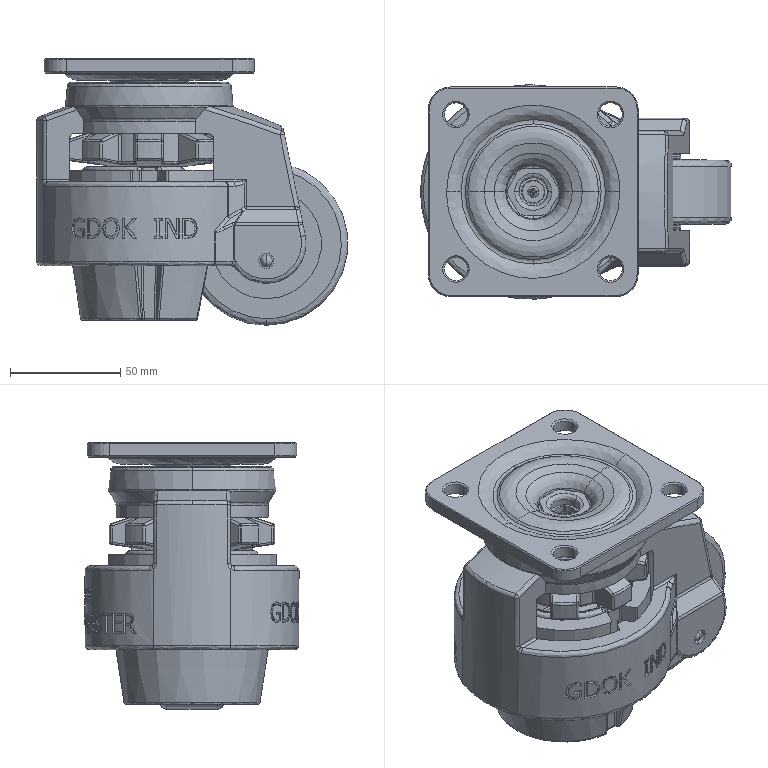Part | SolidWorks | 8 solids | 1732 faces | box 141 x 97.04 x 120.76 mm | volume 659817 mm3 | spline 653 | plane 469 | cylinder 357 | cone 195 | torus 52 | sphere 6 | commonest cylinder face diameters 2 x104 4 x51 98.54 x24 1 x22 12 x12 100.54 x12